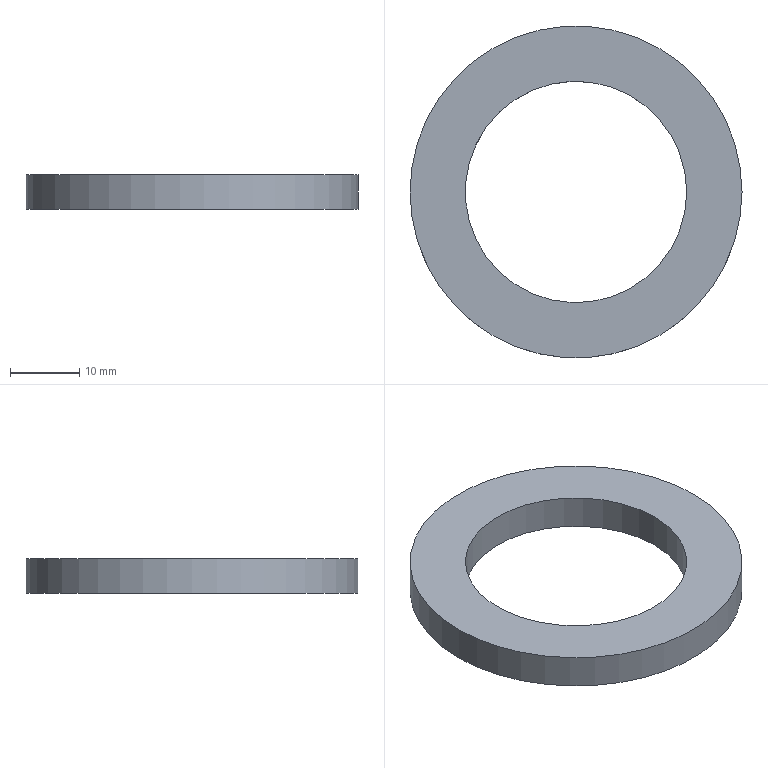Part | NX | features solid 2 | 1 solid | 4 faces | box 48 x 48 x 5 mm | volume 5027 mm3 | cylinder 2 | plane 2 | commonest cylinder face diameters 32 x1 48 x1
STEP:
#1=CARTESIAN_POINT('',(16.,-155.,-70.));
#2=VERTEX_POINT('',#1);
#3=CARTESIAN_POINT('',(0.,-155.,-70.));
#4=DIRECTION('',(0.,0.,1.));
#5=DIRECTION('',(1.,0.,0.));
#6=AXIS2_PLACEMENT_3D('',#3,#4,#5);
#7=CIRCLE('',#6,16.);
#8=EDGE_CURVE('',#2,#2,#7,.T.);
#9=ORIENTED_EDGE('',*,*,#8,.T.);
#10=EDGE_LOOP('',(#9));
#11=FACE_BOUND('',#10,.T.);
#12=CARTESIAN_POINT('',(16.,-155.,-75.));
#13=VERTEX_POINT('',#12);
#14=CARTESIAN_POINT('',(0.,-155.,-75.));
#15=DIRECTION('',(0.,0.,1.));
#16=DIRECTION('',(1.,0.,0.));
#17=AXIS2_PLACEMENT_3D('',#14,#15,#16);
#18=CIRCLE('',#17,16.);
#19=EDGE_CURVE('',#13,#13,#18,.T.);
#20=ORIENTED_EDGE('',*,*,#19,.F.);
#21=EDGE_LOOP('',(#20));
#22=FACE_BOUND('',#21,.T.);
#23=CARTESIAN_POINT('',(0.,-155.,-70.));
#24=DIRECTION('',(0.,0.,-1.));
#25=DIRECTION('',(-1.,0.,0.));
#26=AXIS2_PLACEMENT_3D('',#23,#24,#25);
#27=CYLINDRICAL_SURFACE('',#26,16.);
#28=ADVANCED_FACE('',(#11,#22),#27,.F.);
#29=CARTESIAN_POINT('',(24.,-155.,-70.));
#30=VERTEX_POINT('',#29);
#31=CARTESIAN_POINT('',(0.,-155.,-70.));
#32=DIRECTION('',(0.,0.,1.));
#33=DIRECTION('',(1.,0.,0.));
#34=AXIS2_PLACEMENT_3D('',#31,#32,#33);
#35=CIRCLE('',#34,24.);
#36=EDGE_CURVE('',#30,#30,#35,.T.);
#37=ORIENTED_EDGE('',*,*,#36,.F.);
#38=EDGE_LOOP('',(#37));
#39=FACE_BOUND('',#38,.T.);
#40=CARTESIAN_POINT('',(24.,-155.,-75.));
#41=VERTEX_POINT('',#40);
#42=CARTESIAN_POINT('',(0.,-155.,-75.));
#43=DIRECTION('',(0.,0.,1.));
#44=DIRECTION('',(1.,0.,0.));
#45=AXIS2_PLACEMENT_3D('',#42,#43,#44);
#46=CIRCLE('',#45,24.);
#47=EDGE_CURVE('',#41,#41,#46,.T.);
#48=ORIENTED_EDGE('',*,*,#47,.T.);
#49=EDGE_LOOP('',(#48));
#50=FACE_BOUND('',#49,.T.);
#51=CARTESIAN_POINT('',(0.,-155.,-70.));
#52=DIRECTION('',(0.,0.,-1.));
#53=DIRECTION('',(-1.,0.,0.));
#54=AXIS2_PLACEMENT_3D('',#51,#52,#53);
#55=CYLINDRICAL_SURFACE('',#54,24.);
#56=ADVANCED_FACE('',(#39,#50),#55,.T.);
#57=ORIENTED_EDGE('',*,*,#8,.F.);
#58=EDGE_LOOP('',(#57));
#59=FACE_BOUND('',#58,.T.);
#60=ORIENTED_EDGE('',*,*,#36,.T.);
#61=EDGE_LOOP('',(#60));
#62=FACE_BOUND('',#61,.T.);
#63=CARTESIAN_POINT('',(0.,-155.,-70.));
#64=DIRECTION('',(0.,0.,1.));
#65=DIRECTION('',(1.,0.,0.));
#66=AXIS2_PLACEMENT_3D('',#63,#64,#65);
#67=PLANE('',#66);
#68=ADVANCED_FACE('',(#59,#62),#67,.T.);
#69=ORIENTED_EDGE('',*,*,#19,.T.);
#70=EDGE_LOOP('',(#69));
#71=FACE_BOUND('',#70,.T.);
#72=ORIENTED_EDGE('',*,*,#47,.F.);
#73=EDGE_LOOP('',(#72));
#74=FACE_BOUND('',#73,.T.);
#75=CARTESIAN_POINT('',(0.,-155.,-75.));
#76=DIRECTION('',(0.,0.,1.));
#77=DIRECTION('',(1.,0.,0.));
#78=AXIS2_PLACEMENT_3D('',#75,#76,#77);
#79=PLANE('',#78);
#80=ADVANCED_FACE('',(#71,#74),#79,.F.);
#81=CLOSED_SHELL('',(#28,#56,#68,#80));
#82=MANIFOLD_SOLID_BREP('',#81);
#83=(LENGTH_UNIT()NAMED_UNIT(*)SI_UNIT(.MILLI.,.METRE.));
#84=UNCERTAINTY_MEASURE_WITH_UNIT(LENGTH_MEASURE(0.00001),#83,'','');
#85=(NAMED_UNIT(*)PLANE_ANGLE_UNIT()SI_UNIT($,.RADIAN.));
#86=(NAMED_UNIT(*)SI_UNIT($,.STERADIAN.)SOLID_ANGLE_UNIT());
#87=(GEOMETRIC_REPRESENTATION_CONTEXT(3)GLOBAL_UNCERTAINTY_ASSIGNED_CONTEXT((#84))GLOBAL_UNIT_ASSIGNED_CONTEXT((#83,#85,#86))REPRESENTATION_CONTEXT('',''));
#88=ADVANCED_BREP_SHAPE_REPRESENTATION('',(#82),#87);